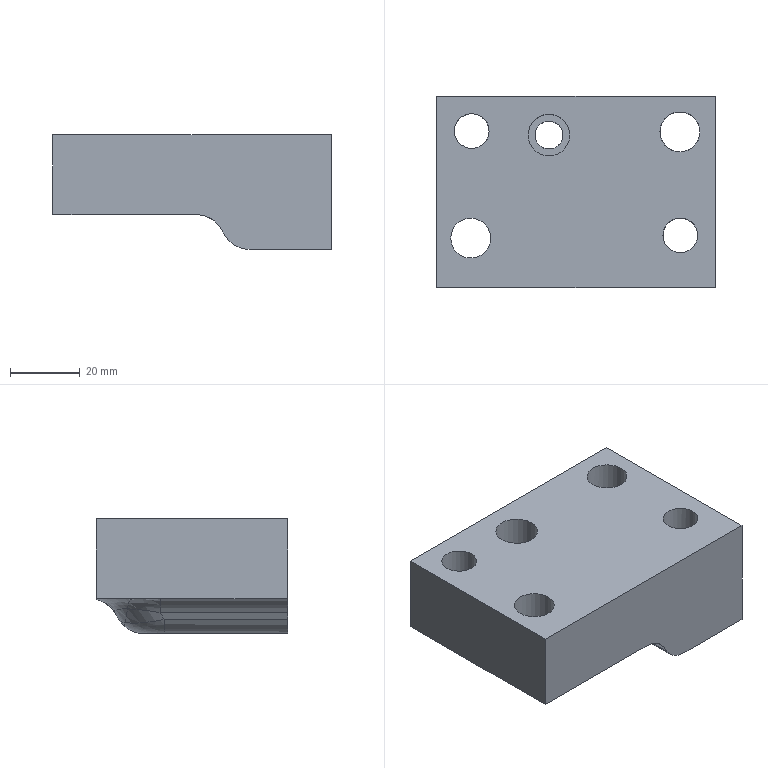Part | NX | features solid 2 | 1 solid | 33 faces | box 80.001 x 55.005 x 33 mm | volume 99625 mm3 | spline 17 | plane 8 | cylinder 8 | commonest cylinder face diameters 10 x2 11.5 x2 17.5 x2 8 x1 12 x1